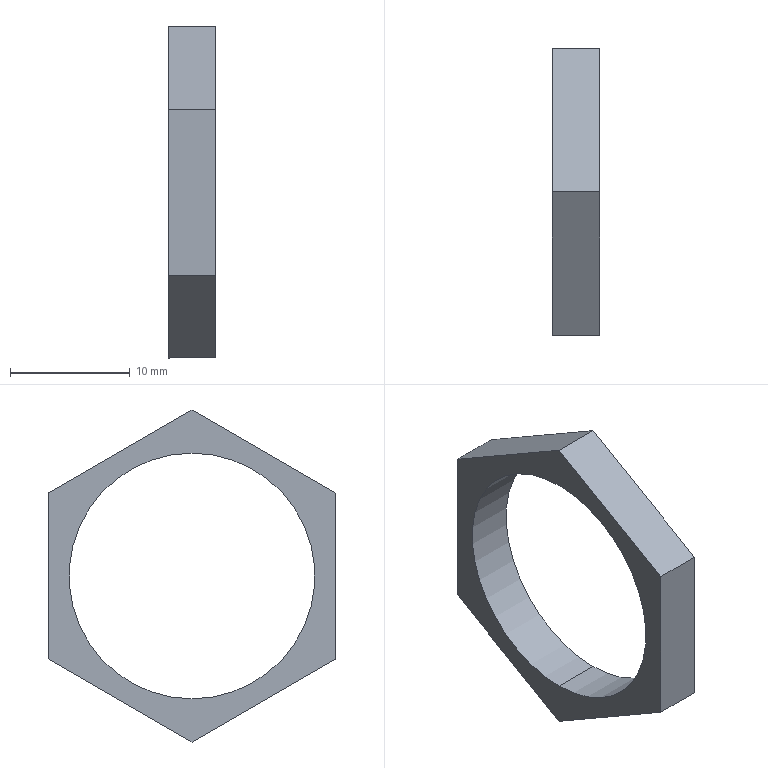Part | SolidWorks | features BaseBody 1 | 1 solid | 10 faces | box 4 x 24 x 27.713 mm | volume 675.068 mm3 | plane 8 | cylinder 2 | commonest cylinder face diameters 20.5 x2
STEP:
#1=CARTESIAN_POINT('',(327.1,95.5,13.25));
#2=VERTEX_POINT('',#1);
#3=CARTESIAN_POINT('',(327.1,95.5,33.75));
#4=VERTEX_POINT('',#3);
#5=CARTESIAN_POINT('',(327.1,95.5,23.5));
#6=DIRECTION('',(-1.,0.,0.));
#7=DIRECTION('',(0.,0.,1.));
#8=AXIS2_PLACEMENT_3D('',#5,#6,#7);
#9=CIRCLE('',#8,10.25);
#10=EDGE_CURVE('',#2,#4,#9,.T.);
#11=ORIENTED_EDGE('',*,*,#10,.F.);
#12=CARTESIAN_POINT('',(323.1,95.5,13.25));
#13=VERTEX_POINT('',#12);
#14=CARTESIAN_POINT('',(327.1,95.5,13.25));
#15=DIRECTION('',(-1.,0.,0.));
#16=VECTOR('',#15,1000.);
#17=LINE('',#14,#16);
#18=EDGE_CURVE('',#2,#13,#17,.T.);
#19=ORIENTED_EDGE('',*,*,#18,.T.);
#20=CARTESIAN_POINT('',(323.1,95.5,33.75));
#21=VERTEX_POINT('',#20);
#22=CARTESIAN_POINT('',(323.1,95.5,23.5));
#23=DIRECTION('',(1.,0.,0.));
#24=DIRECTION('',(0.,0.,1.));
#25=AXIS2_PLACEMENT_3D('',#22,#23,#24);
#26=CIRCLE('',#25,10.25);
#27=EDGE_CURVE('',#21,#13,#26,.T.);
#28=ORIENTED_EDGE('',*,*,#27,.F.);
#29=CARTESIAN_POINT('',(327.1,95.5,33.75));
#30=DIRECTION('',(-1.,0.,0.));
#31=VECTOR('',#30,1000.);
#32=LINE('',#29,#31);
#33=EDGE_CURVE('',#4,#21,#32,.T.);
#34=ORIENTED_EDGE('',*,*,#33,.F.);
#35=EDGE_LOOP('',(#11,#19,#28,#34));
#36=FACE_OUTER_BOUND('',#35,.T.);
#37=CARTESIAN_POINT('',(327.1,95.5,23.5));
#38=DIRECTION('',(-1.,0.,0.));
#39=DIRECTION('',(0.,0.,1.));
#40=AXIS2_PLACEMENT_3D('',#37,#38,#39);
#41=CYLINDRICAL_SURFACE('',#40,10.25);
#42=ADVANCED_FACE('',(#36),#41,.F.);
#43=ORIENTED_EDGE('',*,*,#27,.T.);
#44=CARTESIAN_POINT('',(323.1,95.5,23.5));
#45=DIRECTION('',(1.,0.,0.));
#46=DIRECTION('',(0.,0.,1.));
#47=AXIS2_PLACEMENT_3D('',#44,#45,#46);
#48=CIRCLE('',#47,10.25);
#49=EDGE_CURVE('',#13,#21,#48,.T.);
#50=ORIENTED_EDGE('',*,*,#49,.T.);
#51=EDGE_LOOP('',(#43,#50));
#52=FACE_BOUND('',#51,.T.);
#53=CARTESIAN_POINT('',(323.1,107.5,16.572));
#54=VERTEX_POINT('',#53);
#55=CARTESIAN_POINT('',(323.1,95.5,9.644));
#56=VERTEX_POINT('',#55);
#57=CARTESIAN_POINT('',(323.1,95.5,9.644));
#58=DIRECTION('',(0.,-0.866,-0.5));
#59=VECTOR('',#58,1000.);
#60=LINE('',#57,#59);
#61=EDGE_CURVE('',#54,#56,#60,.T.);
#62=ORIENTED_EDGE('',*,*,#61,.T.);
#63=CARTESIAN_POINT('',(323.1,83.5,16.572));
#64=VERTEX_POINT('',#63);
#65=CARTESIAN_POINT('',(323.1,83.5,16.572));
#66=DIRECTION('',(0.,-0.866,0.5));
#67=VECTOR('',#66,1000.);
#68=LINE('',#65,#67);
#69=EDGE_CURVE('',#56,#64,#68,.T.);
#70=ORIENTED_EDGE('',*,*,#69,.T.);
#71=CARTESIAN_POINT('',(323.1,83.5,30.428));
#72=VERTEX_POINT('',#71);
#73=CARTESIAN_POINT('',(323.1,83.5,16.572));
#74=DIRECTION('',(0.,0.,-1.));
#75=VECTOR('',#74,1000.);
#76=LINE('',#73,#75);
#77=EDGE_CURVE('',#72,#64,#76,.T.);
#78=ORIENTED_EDGE('',*,*,#77,.F.);
#79=CARTESIAN_POINT('',(323.1,95.5,37.356));
#80=VERTEX_POINT('',#79);
#81=CARTESIAN_POINT('',(323.1,95.5,37.356));
#82=DIRECTION('',(0.,0.866,0.5));
#83=VECTOR('',#82,1000.);
#84=LINE('',#81,#83);
#85=EDGE_CURVE('',#72,#80,#84,.T.);
#86=ORIENTED_EDGE('',*,*,#85,.T.);
#87=CARTESIAN_POINT('',(323.1,107.5,30.428));
#88=VERTEX_POINT('',#87);
#89=CARTESIAN_POINT('',(323.1,107.5,30.428));
#90=DIRECTION('',(0.,0.866,-0.5));
#91=VECTOR('',#90,1000.);
#92=LINE('',#89,#91);
#93=EDGE_CURVE('',#80,#88,#92,.T.);
#94=ORIENTED_EDGE('',*,*,#93,.T.);
#95=CARTESIAN_POINT('',(323.1,107.5,30.428));
#96=DIRECTION('',(0.,0.,1.));
#97=VECTOR('',#96,1000.);
#98=LINE('',#95,#97);
#99=EDGE_CURVE('',#54,#88,#98,.T.);
#100=ORIENTED_EDGE('',*,*,#99,.F.);
#101=EDGE_LOOP('',(#62,#70,#78,#86,#94,#100));
#102=FACE_OUTER_BOUND('',#101,.T.);
#103=CARTESIAN_POINT('',(323.1,95.5,23.5));
#104=DIRECTION('',(1.,0.,0.));
#105=DIRECTION('',(0.,1.,0.));
#106=AXIS2_PLACEMENT_3D('',#103,#104,#105);
#107=PLANE('',#106);
#108=ADVANCED_FACE('',(#52,#102),#107,.F.);
#109=CARTESIAN_POINT('',(327.1,95.5,9.644));
#110=VERTEX_POINT('',#109);
#111=CARTESIAN_POINT('',(327.1,107.5,16.572));
#112=VERTEX_POINT('',#111);
#113=CARTESIAN_POINT('',(327.1,95.5,9.644));
#114=DIRECTION('',(0.,0.866,0.5));
#115=VECTOR('',#114,1000.);
#116=LINE('',#113,#115);
#117=EDGE_CURVE('',#110,#112,#116,.T.);
#118=ORIENTED_EDGE('',*,*,#117,.F.);
#119=CARTESIAN_POINT('',(327.1,95.5,9.644));
#120=DIRECTION('',(-1.,0.,0.));
#121=VECTOR('',#120,1000.);
#122=LINE('',#119,#121);
#123=EDGE_CURVE('',#110,#56,#122,.T.);
#124=ORIENTED_EDGE('',*,*,#123,.T.);
#125=ORIENTED_EDGE('',*,*,#61,.F.);
#126=CARTESIAN_POINT('',(327.1,107.5,16.572));
#127=DIRECTION('',(-1.,0.,0.));
#128=VECTOR('',#127,1000.);
#129=LINE('',#126,#128);
#130=EDGE_CURVE('',#112,#54,#129,.T.);
#131=ORIENTED_EDGE('',*,*,#130,.F.);
#132=EDGE_LOOP('',(#118,#124,#125,#131));
#133=FACE_OUTER_BOUND('',#132,.T.);
#134=CARTESIAN_POINT('',(327.1,95.5,9.644));
#135=DIRECTION('',(0.,-0.5,0.866));
#136=DIRECTION('',(-1.,0.,0.));
#137=AXIS2_PLACEMENT_3D('',#134,#135,#136);
#138=PLANE('',#137);
#139=ADVANCED_FACE('',(#133),#138,.F.);
#140=ORIENTED_EDGE('',*,*,#99,.T.);
#141=CARTESIAN_POINT('',(327.1,107.5,30.428));
#142=VERTEX_POINT('',#141);
#143=CARTESIAN_POINT('',(327.1,107.5,30.428));
#144=DIRECTION('',(1.,0.,0.));
#145=VECTOR('',#144,1000.);
#146=LINE('',#143,#145);
#147=EDGE_CURVE('',#88,#142,#146,.T.);
#148=ORIENTED_EDGE('',*,*,#147,.T.);
#149=CARTESIAN_POINT('',(327.1,107.5,23.5));
#150=DIRECTION('',(0.,0.,1.));
#151=VECTOR('',#150,1000.);
#152=LINE('',#149,#151);
#153=EDGE_CURVE('',#112,#142,#152,.T.);
#154=ORIENTED_EDGE('',*,*,#153,.F.);
#155=ORIENTED_EDGE('',*,*,#130,.T.);
#156=EDGE_LOOP('',(#140,#148,#154,#155));
#157=FACE_OUTER_BOUND('',#156,.T.);
#158=CARTESIAN_POINT('',(327.1,107.5,30.428));
#159=DIRECTION('',(0.,1.,0.));
#160=DIRECTION('',(1.,0.,0.));
#161=AXIS2_PLACEMENT_3D('',#158,#159,#160);
#162=PLANE('',#161);
#163=ADVANCED_FACE('',(#157),#162,.T.);
#164=CARTESIAN_POINT('',(327.1,95.5,37.356));
#165=VERTEX_POINT('',#164);
#166=CARTESIAN_POINT('',(327.1,107.5,30.428));
#167=DIRECTION('',(0.,-0.866,0.5));
#168=VECTOR('',#167,1000.);
#169=LINE('',#166,#168);
#170=EDGE_CURVE('',#142,#165,#169,.T.);
#171=ORIENTED_EDGE('',*,*,#170,.F.);
#172=ORIENTED_EDGE('',*,*,#147,.F.);
#173=ORIENTED_EDGE('',*,*,#93,.F.);
#174=CARTESIAN_POINT('',(327.1,95.5,37.356));
#175=DIRECTION('',(1.,0.,0.));
#176=VECTOR('',#175,1000.);
#177=LINE('',#174,#176);
#178=EDGE_CURVE('',#80,#165,#177,.T.);
#179=ORIENTED_EDGE('',*,*,#178,.T.);
#180=EDGE_LOOP('',(#171,#172,#173,#179));
#181=FACE_OUTER_BOUND('',#180,.T.);
#182=CARTESIAN_POINT('',(327.1,107.5,30.428));
#183=DIRECTION('',(0.,-0.5,-0.866));
#184=DIRECTION('',(0.,-0.866,0.5));
#185=AXIS2_PLACEMENT_3D('',#182,#183,#184);
#186=PLANE('',#185);
#187=ADVANCED_FACE('',(#181),#186,.F.);
#188=CARTESIAN_POINT('',(327.1,83.5,30.428));
#189=VERTEX_POINT('',#188);
#190=CARTESIAN_POINT('',(327.1,95.5,37.356));
#191=DIRECTION('',(0.,-0.866,-0.5));
#192=VECTOR('',#191,1000.);
#193=LINE('',#190,#192);
#194=EDGE_CURVE('',#165,#189,#193,.T.);
#195=ORIENTED_EDGE('',*,*,#194,.F.);
#196=ORIENTED_EDGE('',*,*,#178,.F.);
#197=ORIENTED_EDGE('',*,*,#85,.F.);
#198=CARTESIAN_POINT('',(327.1,83.5,30.428));
#199=DIRECTION('',(-1.,0.,0.));
#200=VECTOR('',#199,1000.);
#201=LINE('',#198,#200);
#202=EDGE_CURVE('',#189,#72,#201,.T.);
#203=ORIENTED_EDGE('',*,*,#202,.F.);
#204=EDGE_LOOP('',(#195,#196,#197,#203));
#205=FACE_OUTER_BOUND('',#204,.T.);
#206=CARTESIAN_POINT('',(327.1,95.5,37.356));
#207=DIRECTION('',(0.,0.5,-0.866));
#208=DIRECTION('',(-1.,0.,0.));
#209=AXIS2_PLACEMENT_3D('',#206,#207,#208);
#210=PLANE('',#209);
#211=ADVANCED_FACE('',(#205),#210,.F.);
#212=ORIENTED_EDGE('',*,*,#77,.T.);
#213=CARTESIAN_POINT('',(327.1,83.5,16.572));
#214=VERTEX_POINT('',#213);
#215=CARTESIAN_POINT('',(327.1,83.5,16.572));
#216=DIRECTION('',(1.,0.,0.));
#217=VECTOR('',#216,1000.);
#218=LINE('',#215,#217);
#219=EDGE_CURVE('',#64,#214,#218,.T.);
#220=ORIENTED_EDGE('',*,*,#219,.T.);
#221=CARTESIAN_POINT('',(327.1,83.5,23.5));
#222=DIRECTION('',(0.,0.,-1.));
#223=VECTOR('',#222,1000.);
#224=LINE('',#221,#223);
#225=EDGE_CURVE('',#189,#214,#224,.T.);
#226=ORIENTED_EDGE('',*,*,#225,.F.);
#227=ORIENTED_EDGE('',*,*,#202,.T.);
#228=EDGE_LOOP('',(#212,#220,#226,#227));
#229=FACE_OUTER_BOUND('',#228,.T.);
#230=CARTESIAN_POINT('',(327.1,83.5,16.572));
#231=DIRECTION('',(0.,-1.,0.));
#232=DIRECTION('',(0.,0.,-1.));
#233=AXIS2_PLACEMENT_3D('',#230,#231,#232);
#234=PLANE('',#233);
#235=ADVANCED_FACE('',(#229),#234,.T.);
#236=CARTESIAN_POINT('',(327.1,83.5,16.572));
#237=DIRECTION('',(0.,0.866,-0.5));
#238=VECTOR('',#237,1000.);
#239=LINE('',#236,#238);
#240=EDGE_CURVE('',#214,#110,#239,.T.);
#241=ORIENTED_EDGE('',*,*,#240,.F.);
#242=ORIENTED_EDGE('',*,*,#219,.F.);
#243=ORIENTED_EDGE('',*,*,#69,.F.);
#244=ORIENTED_EDGE('',*,*,#123,.F.);
#245=EDGE_LOOP('',(#241,#242,#243,#244));
#246=FACE_OUTER_BOUND('',#245,.T.);
#247=CARTESIAN_POINT('',(327.1,83.5,16.572));
#248=DIRECTION('',(0.,0.5,0.866));
#249=DIRECTION('',(1.,0.,0.));
#250=AXIS2_PLACEMENT_3D('',#247,#248,#249);
#251=PLANE('',#250);
#252=ADVANCED_FACE('',(#246),#251,.F.);
#253=CARTESIAN_POINT('',(327.1,95.5,23.5));
#254=DIRECTION('',(-1.,0.,0.));
#255=DIRECTION('',(0.,0.,1.));
#256=AXIS2_PLACEMENT_3D('',#253,#254,#255);
#257=CIRCLE('',#256,10.25);
#258=EDGE_CURVE('',#4,#2,#257,.T.);
#259=ORIENTED_EDGE('',*,*,#258,.T.);
#260=ORIENTED_EDGE('',*,*,#10,.T.);
#261=EDGE_LOOP('',(#259,#260));
#262=FACE_BOUND('',#261,.T.);
#263=ORIENTED_EDGE('',*,*,#225,.T.);
#264=ORIENTED_EDGE('',*,*,#240,.T.);
#265=ORIENTED_EDGE('',*,*,#117,.T.);
#266=ORIENTED_EDGE('',*,*,#153,.T.);
#267=ORIENTED_EDGE('',*,*,#170,.T.);
#268=ORIENTED_EDGE('',*,*,#194,.T.);
#269=EDGE_LOOP('',(#263,#264,#265,#266,#267,#268));
#270=FACE_OUTER_BOUND('',#269,.T.);
#271=CARTESIAN_POINT('',(327.1,95.5,23.5));
#272=DIRECTION('',(1.,0.,0.));
#273=DIRECTION('',(0.,1.,0.));
#274=AXIS2_PLACEMENT_3D('',#271,#272,#273);
#275=PLANE('',#274);
#276=ADVANCED_FACE('',(#262,#270),#275,.T.);
#277=ORIENTED_EDGE('',*,*,#18,.F.);
#278=ORIENTED_EDGE('',*,*,#258,.F.);
#279=ORIENTED_EDGE('',*,*,#33,.T.);
#280=ORIENTED_EDGE('',*,*,#49,.F.);
#281=EDGE_LOOP('',(#277,#278,#279,#280));
#282=FACE_OUTER_BOUND('',#281,.T.);
#283=CARTESIAN_POINT('',(327.1,95.5,23.5));
#284=DIRECTION('',(-1.,0.,0.));
#285=DIRECTION('',(0.,0.,1.));
#286=AXIS2_PLACEMENT_3D('',#283,#284,#285);
#287=CYLINDRICAL_SURFACE('',#286,10.25);
#288=ADVANCED_FACE('',(#282),#287,.F.);
#289=CLOSED_SHELL('',(#42,#108,#139,#163,#187,#211,#235,#252,#276,#288));
#290=MANIFOLD_SOLID_BREP('',#289);
#291=CARTESIAN_POINT('',(0.,0.,0.));
#292=DIRECTION('',(0.,0.,1.));
#293=DIRECTION('',(1.,0.,0.));
#294=AXIS2_PLACEMENT_3D('',#291,#292,#293);
#295=(LENGTH_UNIT()NAMED_UNIT(*)SI_UNIT(.MILLI.,.METRE.));
#296=UNCERTAINTY_MEASURE_WITH_UNIT(LENGTH_MEASURE(0.00001),#295,'','');
#297=(NAMED_UNIT(*)PLANE_ANGLE_UNIT()SI_UNIT($,.RADIAN.));
#298=(NAMED_UNIT(*)SI_UNIT($,.STERADIAN.)SOLID_ANGLE_UNIT());
#299=(GEOMETRIC_REPRESENTATION_CONTEXT(3)GLOBAL_UNCERTAINTY_ASSIGNED_CONTEXT((#296))GLOBAL_UNIT_ASSIGNED_CONTEXT((#295,#297,#298))REPRESENTATION_CONTEXT('',''));
#300=ADVANCED_BREP_SHAPE_REPRESENTATION('',(#290,#294),#299);